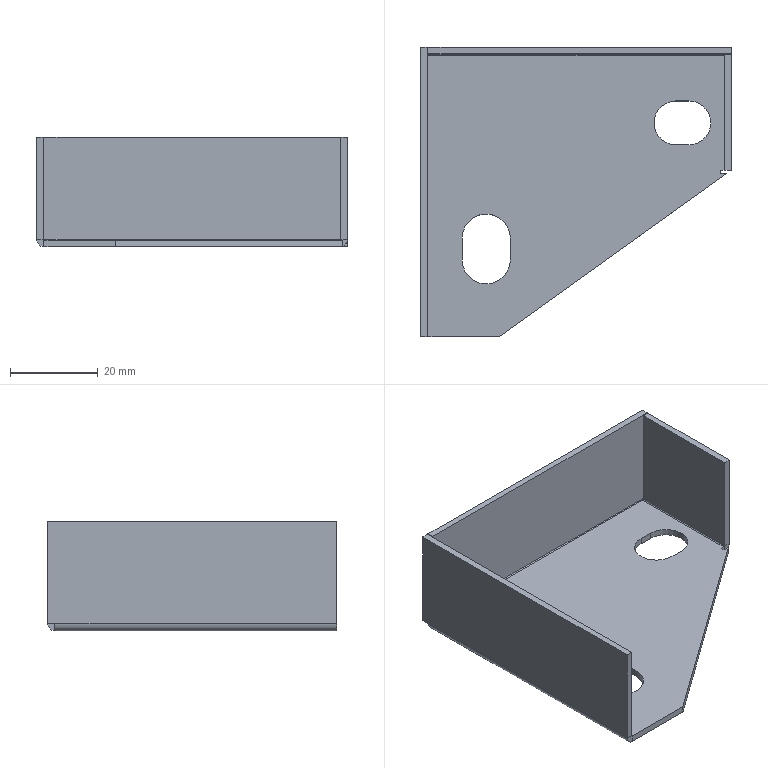Part | 1 solid | 45 faces | box 71 x 66 x 25 mm | volume 10722 mm3 | plane 34 | cylinder 11 | commonest cylinder face diameters 0.4 x3 3.4 x3 10 x3 11 x2
STEP:
#1=CARTESIAN_POINT('',(30.8,15.8,-1.5));
#2=VERTEX_POINT('',#1);
#3=CARTESIAN_POINT('',(25.8,20.8,-1.5));
#4=VERTEX_POINT('',#3);
#5=CARTESIAN_POINT('',(25.8,15.8,-1.5));
#6=DIRECTION('',(0.,0.,1.));
#7=DIRECTION('',(1.,0.,0.));
#8=AXIS2_PLACEMENT_3D('',#5,#6,#7);
#9=CIRCLE('',#8,5.);
#10=EDGE_CURVE('',#2,#4,#9,.T.);
#11=ORIENTED_EDGE('',*,*,#10,.F.);
#12=CARTESIAN_POINT('',(30.8,15.8,0.));
#13=VERTEX_POINT('',#12);
#14=CARTESIAN_POINT('',(30.8,15.8,-10.));
#15=DIRECTION('',(0.,0.,1.));
#16=VECTOR('',#15,1000.);
#17=LINE('',#14,#16);
#18=EDGE_CURVE('',#2,#13,#17,.T.);
#19=ORIENTED_EDGE('',*,*,#18,.T.);
#20=CARTESIAN_POINT('',(25.8,20.8,0.));
#21=VERTEX_POINT('',#20);
#22=CARTESIAN_POINT('',(25.8,15.8,0.));
#23=DIRECTION('',(0.,0.,1.));
#24=DIRECTION('',(1.,0.,0.));
#25=AXIS2_PLACEMENT_3D('',#22,#23,#24);
#26=CIRCLE('',#25,5.);
#27=EDGE_CURVE('',#13,#21,#26,.T.);
#28=ORIENTED_EDGE('',*,*,#27,.T.);
#29=CARTESIAN_POINT('',(25.8,20.8,-10.));
#30=DIRECTION('',(0.,0.,1.));
#31=VECTOR('',#30,1000.);
#32=LINE('',#29,#31);
#33=EDGE_CURVE('',#4,#21,#32,.T.);
#34=ORIENTED_EDGE('',*,*,#33,.F.);
#35=EDGE_LOOP('',(#11,#19,#28,#34));
#36=FACE_OUTER_BOUND('',#35,.T.);
#37=CARTESIAN_POINT('',(25.8,15.8,-10.));
#38=DIRECTION('',(0.,0.,1.));
#39=DIRECTION('',(1.,0.,0.));
#40=AXIS2_PLACEMENT_3D('',#37,#38,#39);
#41=CYLINDRICAL_SURFACE('',#40,5.);
#42=ADVANCED_FACE('',(#36),#41,.F.);
#43=CARTESIAN_POINT('',(35.5,31.3,0.));
#44=VERTEX_POINT('',#43);
#45=CARTESIAN_POINT('',(35.488,31.3,0.));
#46=VERTEX_POINT('',#45);
#47=CARTESIAN_POINT('',(35.5,31.3,0.));
#48=DIRECTION('',(-1.,0.,0.));
#49=VECTOR('',#48,1000.);
#50=LINE('',#47,#49);
#51=EDGE_CURVE('',#44,#46,#50,.T.);
#52=ORIENTED_EDGE('',*,*,#51,.T.);
#53=CARTESIAN_POINT('',(33.8,31.3,-1.5));
#54=VERTEX_POINT('',#53);
#55=CARTESIAN_POINT('',(33.8,31.3,0.2));
#56=DIRECTION('',(0.,1.,0.));
#57=DIRECTION('',(0.,0.,1.));
#58=AXIS2_PLACEMENT_3D('',#55,#56,#57);
#59=CIRCLE('',#58,1.7);
#60=EDGE_CURVE('',#46,#54,#59,.T.);
#61=ORIENTED_EDGE('',*,*,#60,.T.);
#62=CARTESIAN_POINT('',(35.5,31.3,-1.5));
#63=VERTEX_POINT('',#62);
#64=CARTESIAN_POINT('',(-33.8,31.3,-1.5));
#65=DIRECTION('',(-1.,0.,0.));
#66=VECTOR('',#65,1000.);
#67=LINE('',#64,#66);
#68=EDGE_CURVE('',#63,#54,#67,.T.);
#69=ORIENTED_EDGE('',*,*,#68,.F.);
#70=CARTESIAN_POINT('',(35.5,31.3,0.));
#71=DIRECTION('',(0.,0.,-1.));
#72=VECTOR('',#71,1000.);
#73=LINE('',#70,#72);
#74=EDGE_CURVE('',#44,#63,#73,.T.);
#75=ORIENTED_EDGE('',*,*,#74,.F.);
#76=EDGE_LOOP('',(#52,#61,#69,#75));
#77=FACE_OUTER_BOUND('',#76,.T.);
#78=CARTESIAN_POINT('',(35.5,31.3,0.));
#79=DIRECTION('',(0.,-1.,0.));
#80=DIRECTION('',(0.,0.,-1.));
#81=AXIS2_PLACEMENT_3D('',#78,#79,#80);
#82=PLANE('',#81);
#83=ADVANCED_FACE('',(#77),#82,.T.);
#84=CARTESIAN_POINT('',(-15.,-15.5,-1.5));
#85=VERTEX_POINT('',#84);
#86=CARTESIAN_POINT('',(-15.,-10.5,-1.5));
#87=VERTEX_POINT('',#86);
#88=CARTESIAN_POINT('',(-15.,0.,-1.5));
#89=DIRECTION('',(0.,1.,0.));
#90=VECTOR('',#89,1000.);
#91=LINE('',#88,#90);
#92=EDGE_CURVE('',#85,#87,#91,.T.);
#93=ORIENTED_EDGE('',*,*,#92,.T.);
#94=CARTESIAN_POINT('',(-26.,-10.5,-1.5));
#95=VERTEX_POINT('',#94);
#96=CARTESIAN_POINT('',(-20.5,-10.5,-1.5));
#97=DIRECTION('',(0.,0.,1.));
#98=DIRECTION('',(1.,0.,0.));
#99=AXIS2_PLACEMENT_3D('',#96,#97,#98);
#100=CIRCLE('',#99,5.5);
#101=EDGE_CURVE('',#87,#95,#100,.T.);
#102=ORIENTED_EDGE('',*,*,#101,.T.);
#103=CARTESIAN_POINT('',(-26.,-15.5,-1.5));
#104=VERTEX_POINT('',#103);
#105=CARTESIAN_POINT('',(-26.,0.,-1.5));
#106=DIRECTION('',(0.,-1.,0.));
#107=VECTOR('',#106,1000.);
#108=LINE('',#105,#107);
#109=EDGE_CURVE('',#95,#104,#108,.T.);
#110=ORIENTED_EDGE('',*,*,#109,.T.);
#111=CARTESIAN_POINT('',(-20.5,-15.5,-1.5));
#112=DIRECTION('',(0.,0.,1.));
#113=DIRECTION('',(1.,0.,0.));
#114=AXIS2_PLACEMENT_3D('',#111,#112,#113);
#115=CIRCLE('',#114,5.5);
#116=EDGE_CURVE('',#104,#85,#115,.T.);
#117=ORIENTED_EDGE('',*,*,#116,.T.);
#118=EDGE_LOOP('',(#93,#102,#110,#117));
#119=FACE_BOUND('',#118,.T.);
#120=CARTESIAN_POINT('',(22.8,20.8,-1.5));
#121=VERTEX_POINT('',#120);
#122=CARTESIAN_POINT('',(0.,20.8,-1.5));
#123=DIRECTION('',(-1.,0.,0.));
#124=VECTOR('',#123,1000.);
#125=LINE('',#122,#124);
#126=EDGE_CURVE('',#4,#121,#125,.T.);
#127=ORIENTED_EDGE('',*,*,#126,.T.);
#128=CARTESIAN_POINT('',(22.8,10.8,-1.5));
#129=VERTEX_POINT('',#128);
#130=CARTESIAN_POINT('',(22.8,15.8,-1.5));
#131=DIRECTION('',(0.,0.,1.));
#132=DIRECTION('',(1.,0.,0.));
#133=AXIS2_PLACEMENT_3D('',#130,#131,#132);
#134=CIRCLE('',#133,5.);
#135=EDGE_CURVE('',#121,#129,#134,.T.);
#136=ORIENTED_EDGE('',*,*,#135,.T.);
#137=CARTESIAN_POINT('',(25.8,10.8,-1.5));
#138=VERTEX_POINT('',#137);
#139=CARTESIAN_POINT('',(0.,10.8,-1.5));
#140=DIRECTION('',(1.,0.,0.));
#141=VECTOR('',#140,1000.);
#142=LINE('',#139,#141);
#143=EDGE_CURVE('',#129,#138,#142,.T.);
#144=ORIENTED_EDGE('',*,*,#143,.T.);
#145=CARTESIAN_POINT('',(25.8,15.8,-1.5));
#146=DIRECTION('',(0.,0.,1.));
#147=DIRECTION('',(1.,0.,0.));
#148=AXIS2_PLACEMENT_3D('',#145,#146,#147);
#149=CIRCLE('',#148,5.);
#150=EDGE_CURVE('',#138,#2,#149,.T.);
#151=ORIENTED_EDGE('',*,*,#150,.T.);
#152=ORIENTED_EDGE('',*,*,#10,.T.);
#153=EDGE_LOOP('',(#127,#136,#144,#151,#152));
#154=FACE_BOUND('',#153,.T.);
#155=CARTESIAN_POINT('',(33.8,5.,-1.5));
#156=VERTEX_POINT('',#155);
#157=CARTESIAN_POINT('',(33.8,31.3,-1.5));
#158=DIRECTION('',(0.,-1.,0.));
#159=VECTOR('',#158,1000.);
#160=LINE('',#157,#159);
#161=EDGE_CURVE('',#54,#156,#160,.T.);
#162=ORIENTED_EDGE('',*,*,#161,.T.);
#163=CARTESIAN_POINT('',(33.05,5.,-1.5));
#164=VERTEX_POINT('',#163);
#165=CARTESIAN_POINT('',(0.,5.,-1.5));
#166=DIRECTION('',(1.,0.,0.));
#167=VECTOR('',#166,1000.);
#168=LINE('',#165,#167);
#169=EDGE_CURVE('',#164,#156,#168,.T.);
#170=ORIENTED_EDGE('',*,*,#169,.F.);
#171=CARTESIAN_POINT('',(33.05,4.25,-1.5));
#172=VERTEX_POINT('',#171);
#173=CARTESIAN_POINT('',(33.05,0.,-1.5));
#174=DIRECTION('',(0.,1.,0.));
#175=VECTOR('',#174,1000.);
#176=LINE('',#173,#175);
#177=EDGE_CURVE('',#172,#164,#176,.T.);
#178=ORIENTED_EDGE('',*,*,#177,.F.);
#179=CARTESIAN_POINT('',(34.454,4.25,-1.5));
#180=VERTEX_POINT('',#179);
#181=CARTESIAN_POINT('',(0.,4.25,-1.5));
#182=DIRECTION('',(-1.,0.,0.));
#183=VECTOR('',#182,1000.);
#184=LINE('',#181,#183);
#185=EDGE_CURVE('',#180,#172,#184,.T.);
#186=ORIENTED_EDGE('',*,*,#185,.F.);
#187=CARTESIAN_POINT('',(-17.5,-33.,-1.5));
#188=VERTEX_POINT('',#187);
#189=CARTESIAN_POINT('',(9.685,-13.509,-1.5));
#190=DIRECTION('',(-0.8127,-0.5827,0.));
#191=VECTOR('',#190,1000.);
#192=LINE('',#189,#191);
#193=EDGE_CURVE('',#180,#188,#192,.T.);
#194=ORIENTED_EDGE('',*,*,#193,.T.);
#195=CARTESIAN_POINT('',(-33.8,-33.,-1.5));
#196=VERTEX_POINT('',#195);
#197=CARTESIAN_POINT('',(-35.5,-33.,-1.5));
#198=DIRECTION('',(1.,0.,0.));
#199=VECTOR('',#198,1000.);
#200=LINE('',#197,#199);
#201=EDGE_CURVE('',#196,#188,#200,.T.);
#202=ORIENTED_EDGE('',*,*,#201,.F.);
#203=CARTESIAN_POINT('',(-33.8,31.3,-1.5));
#204=VERTEX_POINT('',#203);
#205=CARTESIAN_POINT('',(-33.8,-33.,-1.5));
#206=DIRECTION('',(0.,1.,0.));
#207=VECTOR('',#206,1000.);
#208=LINE('',#205,#207);
#209=EDGE_CURVE('',#196,#204,#208,.T.);
#210=ORIENTED_EDGE('',*,*,#209,.T.);
#211=CARTESIAN_POINT('',(-33.8,31.3,-1.5));
#212=DIRECTION('',(1.,0.,0.));
#213=VECTOR('',#212,1000.);
#214=LINE('',#211,#213);
#215=EDGE_CURVE('',#204,#54,#214,.T.);
#216=ORIENTED_EDGE('',*,*,#215,.T.);
#217=EDGE_LOOP('',(#162,#170,#178,#186,#194,#202,#210,#216));
#218=FACE_OUTER_BOUND('',#217,.T.);
#219=CARTESIAN_POINT('',(0.,0.,-1.5));
#220=DIRECTION('',(0.,0.,1.));
#221=DIRECTION('',(1.,0.,0.));
#222=AXIS2_PLACEMENT_3D('',#219,#220,#221);
#223=PLANE('',#222);
#224=ADVANCED_FACE('',(#119,#154,#218),#223,.F.);
#225=CARTESIAN_POINT('',(22.8,20.8,0.));
#226=VERTEX_POINT('',#225);
#227=CARTESIAN_POINT('',(22.8,10.8,0.));
#228=VERTEX_POINT('',#227);
#229=CARTESIAN_POINT('',(22.8,15.8,0.));
#230=DIRECTION('',(0.,0.,1.));
#231=DIRECTION('',(1.,0.,0.));
#232=AXIS2_PLACEMENT_3D('',#229,#230,#231);
#233=CIRCLE('',#232,5.);
#234=EDGE_CURVE('',#226,#228,#233,.T.);
#235=ORIENTED_EDGE('',*,*,#234,.F.);
#236=CARTESIAN_POINT('',(22.8,20.8,0.));
#237=DIRECTION('',(-1.,0.,0.));
#238=VECTOR('',#237,1000.);
#239=LINE('',#236,#238);
#240=EDGE_CURVE('',#21,#226,#239,.T.);
#241=ORIENTED_EDGE('',*,*,#240,.F.);
#242=ORIENTED_EDGE('',*,*,#27,.F.);
#243=CARTESIAN_POINT('',(25.8,10.8,0.));
#244=VERTEX_POINT('',#243);
#245=CARTESIAN_POINT('',(25.8,15.8,0.));
#246=DIRECTION('',(0.,0.,1.));
#247=DIRECTION('',(1.,0.,0.));
#248=AXIS2_PLACEMENT_3D('',#245,#246,#247);
#249=CIRCLE('',#248,5.);
#250=EDGE_CURVE('',#244,#13,#249,.T.);
#251=ORIENTED_EDGE('',*,*,#250,.F.);
#252=CARTESIAN_POINT('',(22.8,10.8,0.));
#253=DIRECTION('',(1.,0.,0.));
#254=VECTOR('',#253,1000.);
#255=LINE('',#252,#254);
#256=EDGE_CURVE('',#228,#244,#255,.T.);
#257=ORIENTED_EDGE('',*,*,#256,.F.);
#258=EDGE_LOOP('',(#235,#241,#242,#251,#257));
#259=FACE_BOUND('',#258,.T.);
#260=CARTESIAN_POINT('',(-15.,-10.5,0.));
#261=VERTEX_POINT('',#260);
#262=CARTESIAN_POINT('',(-26.,-10.5,0.));
#263=VERTEX_POINT('',#262);
#264=CARTESIAN_POINT('',(-20.5,-10.5,0.));
#265=DIRECTION('',(0.,0.,1.));
#266=DIRECTION('',(1.,0.,0.));
#267=AXIS2_PLACEMENT_3D('',#264,#265,#266);
#268=CIRCLE('',#267,5.5);
#269=EDGE_CURVE('',#261,#263,#268,.T.);
#270=ORIENTED_EDGE('',*,*,#269,.F.);
#271=CARTESIAN_POINT('',(-15.,-15.5,0.));
#272=VERTEX_POINT('',#271);
#273=CARTESIAN_POINT('',(-15.,-10.5,0.));
#274=DIRECTION('',(0.,1.,0.));
#275=VECTOR('',#274,1000.);
#276=LINE('',#273,#275);
#277=EDGE_CURVE('',#272,#261,#276,.T.);
#278=ORIENTED_EDGE('',*,*,#277,.F.);
#279=CARTESIAN_POINT('',(-26.,-15.5,0.));
#280=VERTEX_POINT('',#279);
#281=CARTESIAN_POINT('',(-20.5,-15.5,0.));
#282=DIRECTION('',(0.,0.,1.));
#283=DIRECTION('',(1.,0.,0.));
#284=AXIS2_PLACEMENT_3D('',#281,#282,#283);
#285=CIRCLE('',#284,5.5);
#286=EDGE_CURVE('',#280,#272,#285,.T.);
#287=ORIENTED_EDGE('',*,*,#286,.F.);
#288=CARTESIAN_POINT('',(-26.,-10.5,0.));
#289=DIRECTION('',(0.,-1.,0.));
#290=VECTOR('',#289,1000.);
#291=LINE('',#288,#290);
#292=EDGE_CURVE('',#263,#280,#291,.T.);
#293=ORIENTED_EDGE('',*,*,#292,.F.);
#294=EDGE_LOOP('',(#270,#278,#287,#293));
#295=FACE_BOUND('',#294,.T.);
#296=CARTESIAN_POINT('',(33.8,5.,0.));
#297=VERTEX_POINT('',#296);
#298=CARTESIAN_POINT('',(33.05,5.,0.));
#299=VERTEX_POINT('',#298);
#300=CARTESIAN_POINT('',(33.8,5.,0.));
#301=DIRECTION('',(-1.,0.,0.));
#302=VECTOR('',#301,1000.);
#303=LINE('',#300,#302);
#304=EDGE_CURVE('',#297,#299,#303,.T.);
#305=ORIENTED_EDGE('',*,*,#304,.F.);
#306=CARTESIAN_POINT('',(33.8,31.3,0.));
#307=VERTEX_POINT('',#306);
#308=CARTESIAN_POINT('',(33.8,31.3,0.));
#309=DIRECTION('',(0.,-1.,0.));
#310=VECTOR('',#309,1000.);
#311=LINE('',#308,#310);
#312=EDGE_CURVE('',#307,#297,#311,.T.);
#313=ORIENTED_EDGE('',*,*,#312,.F.);
#314=CARTESIAN_POINT('',(-33.8,31.3,0.));
#315=VERTEX_POINT('',#314);
#316=CARTESIAN_POINT('',(-33.8,31.3,0.));
#317=DIRECTION('',(1.,0.,0.));
#318=VECTOR('',#317,1000.);
#319=LINE('',#316,#318);
#320=EDGE_CURVE('',#315,#307,#319,.T.);
#321=ORIENTED_EDGE('',*,*,#320,.F.);
#322=CARTESIAN_POINT('',(-33.8,-33.,0.));
#323=VERTEX_POINT('',#322);
#324=CARTESIAN_POINT('',(-33.8,-33.,0.));
#325=DIRECTION('',(0.,1.,0.));
#326=VECTOR('',#325,1000.);
#327=LINE('',#324,#326);
#328=EDGE_CURVE('',#323,#315,#327,.T.);
#329=ORIENTED_EDGE('',*,*,#328,.F.);
#330=CARTESIAN_POINT('',(-17.5,-33.,0.));
#331=VERTEX_POINT('',#330);
#332=CARTESIAN_POINT('',(-35.5,-33.,0.));
#333=DIRECTION('',(1.,0.,0.));
#334=VECTOR('',#333,1000.);
#335=LINE('',#332,#334);
#336=EDGE_CURVE('',#323,#331,#335,.T.);
#337=ORIENTED_EDGE('',*,*,#336,.T.);
#338=CARTESIAN_POINT('',(34.454,4.25,0.));
#339=VERTEX_POINT('',#338);
#340=CARTESIAN_POINT('',(9.685,-13.509,0.));
#341=DIRECTION('',(-0.8127,-0.5827,0.));
#342=VECTOR('',#341,1000.);
#343=LINE('',#340,#342);
#344=EDGE_CURVE('',#339,#331,#343,.T.);
#345=ORIENTED_EDGE('',*,*,#344,.F.);
#346=CARTESIAN_POINT('',(33.05,4.25,0.));
#347=VERTEX_POINT('',#346);
#348=CARTESIAN_POINT('',(33.05,4.25,0.));
#349=DIRECTION('',(1.,0.,0.));
#350=VECTOR('',#349,1000.);
#351=LINE('',#348,#350);
#352=EDGE_CURVE('',#347,#339,#351,.T.);
#353=ORIENTED_EDGE('',*,*,#352,.F.);
#354=CARTESIAN_POINT('',(33.05,5.,0.));
#355=DIRECTION('',(0.,-1.,0.));
#356=VECTOR('',#355,1000.);
#357=LINE('',#354,#356);
#358=EDGE_CURVE('',#299,#347,#357,.T.);
#359=ORIENTED_EDGE('',*,*,#358,.F.);
#360=EDGE_LOOP('',(#305,#313,#321,#329,#337,#345,#353,#359));
#361=FACE_OUTER_BOUND('',#360,.T.);
#362=CARTESIAN_POINT('',(0.,0.,0.));
#363=DIRECTION('',(0.,0.,1.));
#364=DIRECTION('',(1.,0.,0.));
#365=AXIS2_PLACEMENT_3D('',#362,#363,#364);
#366=PLANE('',#365);
#367=ADVANCED_FACE('',(#259,#295,#361),#366,.T.);
#368=CARTESIAN_POINT('',(34.454,4.25,0.));
#369=DIRECTION('',(0.,0.,-1.));
#370=VECTOR('',#369,1000.);
#371=LINE('',#368,#370);
#372=EDGE_CURVE('',#339,#180,#371,.T.);
#373=ORIENTED_EDGE('',*,*,#372,.F.);
#374=ORIENTED_EDGE('',*,*,#344,.T.);
#375=CARTESIAN_POINT('',(-17.5,-33.,23.5));
#376=DIRECTION('',(0.,0.,-1.));
#377=VECTOR('',#376,1000.);
#378=LINE('',#375,#377);
#379=EDGE_CURVE('',#331,#188,#378,.T.);
#380=ORIENTED_EDGE('',*,*,#379,.T.);
#381=ORIENTED_EDGE('',*,*,#193,.F.);
#382=EDGE_LOOP('',(#373,#374,#380,#381));
#383=FACE_OUTER_BOUND('',#382,.T.);
#384=CARTESIAN_POINT('',(35.5,5.,23.5));
#385=DIRECTION('',(-0.5827,0.8127,0.));
#386=DIRECTION('',(-0.8127,-0.5827,0.));
#387=AXIS2_PLACEMENT_3D('',#384,#385,#386);
#388=PLANE('',#387);
#389=ADVANCED_FACE('',(#383),#388,.F.);
#390=CARTESIAN_POINT('',(-35.5,31.3,0.2));
#391=VERTEX_POINT('',#390);
#392=CARTESIAN_POINT('',(-34.,31.3,0.2));
#393=VERTEX_POINT('',#392);
#394=CARTESIAN_POINT('',(-35.5,31.3,0.2));
#395=DIRECTION('',(1.,0.,0.));
#396=VECTOR('',#395,1000.);
#397=LINE('',#394,#396);
#398=EDGE_CURVE('',#391,#393,#397,.T.);
#399=ORIENTED_EDGE('',*,*,#398,.F.);
#400=CARTESIAN_POINT('',(-35.5,33.,0.2));
#401=VERTEX_POINT('',#400);
#402=CARTESIAN_POINT('',(-35.5,33.,0.2));
#403=DIRECTION('',(0.,1.,0.));
#404=VECTOR('',#403,1000.);
#405=LINE('',#402,#404);
#406=EDGE_CURVE('',#391,#401,#405,.T.);
#407=ORIENTED_EDGE('',*,*,#406,.T.);
#408=CARTESIAN_POINT('',(-34.,33.,0.2));
#409=VERTEX_POINT('',#408);
#410=CARTESIAN_POINT('',(-35.5,33.,0.2));
#411=DIRECTION('',(-1.,0.,0.));
#412=VECTOR('',#411,1000.);
#413=LINE('',#410,#412);
#414=EDGE_CURVE('',#409,#401,#413,.T.);
#415=ORIENTED_EDGE('',*,*,#414,.F.);
#416=CARTESIAN_POINT('',(-34.,33.,0.2));
#417=DIRECTION('',(0.,-1.,0.));
#418=VECTOR('',#417,1000.);
#419=LINE('',#416,#418);
#420=EDGE_CURVE('',#409,#393,#419,.T.);
#421=ORIENTED_EDGE('',*,*,#420,.T.);
#422=EDGE_LOOP('',(#399,#407,#415,#421));
#423=FACE_OUTER_BOUND('',#422,.T.);
#424=CARTESIAN_POINT('',(0.,0.,0.2));
#425=DIRECTION('',(0.,0.,-1.));
#426=DIRECTION('',(-1.,0.,0.));
#427=AXIS2_PLACEMENT_3D('',#424,#425,#426);
#428=PLANE('',#427);
#429=ADVANCED_FACE('',(#423),#428,.T.);
#430=CARTESIAN_POINT('',(-35.5,-33.,0.2));
#431=VERTEX_POINT('',#430);
#432=CARTESIAN_POINT('',(-35.5,33.,0.2));
#433=DIRECTION('',(0.,1.,0.));
#434=VECTOR('',#433,1000.);
#435=LINE('',#432,#434);
#436=EDGE_CURVE('',#431,#391,#435,.T.);
#437=ORIENTED_EDGE('',*,*,#436,.T.);
#438=CARTESIAN_POINT('',(-33.8,31.3,0.2));
#439=DIRECTION('',(0.,-1.,0.));
#440=DIRECTION('',(0.,0.,1.));
#441=AXIS2_PLACEMENT_3D('',#438,#439,#440);
#442=CIRCLE('',#441,1.7);
#443=EDGE_CURVE('',#391,#204,#442,.T.);
#444=ORIENTED_EDGE('',*,*,#443,.T.);
#445=ORIENTED_EDGE('',*,*,#209,.F.);
#446=CARTESIAN_POINT('',(-33.8,-33.,0.2));
#447=DIRECTION('',(0.,-1.,0.));
#448=DIRECTION('',(0.,0.,-1.));
#449=AXIS2_PLACEMENT_3D('',#446,#447,#448);
#450=CIRCLE('',#449,1.7);
#451=EDGE_CURVE('',#431,#196,#450,.T.);
#452=ORIENTED_EDGE('',*,*,#451,.F.);
#453=EDGE_LOOP('',(#437,#444,#445,#452));
#454=FACE_OUTER_BOUND('',#453,.T.);
#455=CARTESIAN_POINT('',(-33.8,-33.,0.2));
#456=DIRECTION('',(0.,-1.,0.));
#457=DIRECTION('',(-1.,0.,0.));
#458=AXIS2_PLACEMENT_3D('',#455,#456,#457);
#459=CYLINDRICAL_SURFACE('',#458,1.7);
#460=ADVANCED_FACE('',(#454),#459,.T.);
#461=ORIENTED_EDGE('',*,*,#379,.F.);
#462=ORIENTED_EDGE('',*,*,#336,.F.);
#463=CARTESIAN_POINT('',(-33.8,-33.,0.));
#464=DIRECTION('',(0.,0.,-1.));
#465=VECTOR('',#464,1000.);
#466=LINE('',#463,#465);
#467=EDGE_CURVE('',#323,#196,#466,.T.);
#468=ORIENTED_EDGE('',*,*,#467,.T.);
#469=ORIENTED_EDGE('',*,*,#201,.T.);
#470=EDGE_LOOP('',(#461,#462,#468,#469));
#471=FACE_OUTER_BOUND('',#470,.T.);
#472=CARTESIAN_POINT('',(-35.5,-33.,-1.5));
#473=DIRECTION('',(0.,-1.,0.));
#474=DIRECTION('',(0.,0.,-1.));
#475=AXIS2_PLACEMENT_3D('',#472,#473,#474);
#476=PLANE('',#475);
#477=ADVANCED_FACE('',(#471),#476,.T.);
#478=CARTESIAN_POINT('',(-15.,-10.5,-10.));
#479=DIRECTION('',(0.,0.,1.));
#480=VECTOR('',#479,1000.);
#481=LINE('',#478,#480);
#482=EDGE_CURVE('',#87,#261,#481,.T.);
#483=ORIENTED_EDGE('',*,*,#482,.T.);
#484=ORIENTED_EDGE('',*,*,#269,.T.);
#485=CARTESIAN_POINT('',(-26.,-10.5,-10.));
#486=DIRECTION('',(0.,0.,1.));
#487=VECTOR('',#486,1000.);
#488=LINE('',#485,#487);
#489=EDGE_CURVE('',#95,#263,#488,.T.);
#490=ORIENTED_EDGE('',*,*,#489,.F.);
#491=ORIENTED_EDGE('',*,*,#101,.F.);
#492=EDGE_LOOP('',(#483,#484,#490,#491));
#493=FACE_OUTER_BOUND('',#492,.T.);
#494=CARTESIAN_POINT('',(-20.5,-10.5,-10.));
#495=DIRECTION('',(0.,0.,1.));
#496=DIRECTION('',(1.,0.,0.));
#497=AXIS2_PLACEMENT_3D('',#494,#495,#496);
#498=CYLINDRICAL_SURFACE('',#497,5.5);
#499=ADVANCED_FACE('',(#493),#498,.F.);
#500=CARTESIAN_POINT('',(-15.,-15.5,-10.));
#501=DIRECTION('',(0.,0.,1.));
#502=VECTOR('',#501,1000.);
#503=LINE('',#500,#502);
#504=EDGE_CURVE('',#85,#272,#503,.T.);
#505=ORIENTED_EDGE('',*,*,#504,.T.);
#506=ORIENTED_EDGE('',*,*,#277,.T.);
#507=ORIENTED_EDGE('',*,*,#482,.F.);
#508=ORIENTED_EDGE('',*,*,#92,.F.);
#509=EDGE_LOOP('',(#505,#506,#507,#508));
#510=FACE_OUTER_BOUND('',#509,.T.);
#511=CARTESIAN_POINT('',(-15.,-10.5,-10.));
#512=DIRECTION('',(1.,0.,0.));
#513=DIRECTION('',(0.,0.,-1.));
#514=AXIS2_PLACEMENT_3D('',#511,#512,#513);
#515=PLANE('',#514);
#516=ADVANCED_FACE('',(#510),#515,.F.);
#517=CARTESIAN_POINT('',(-26.,-15.5,-10.));
#518=DIRECTION('',(0.,0.,1.));
#519=VECTOR('',#518,1000.);
#520=LINE('',#517,#519);
#521=EDGE_CURVE('',#104,#280,#520,.T.);
#522=ORIENTED_EDGE('',*,*,#521,.T.);
#523=ORIENTED_EDGE('',*,*,#286,.T.);
#524=ORIENTED_EDGE('',*,*,#504,.F.);
#525=ORIENTED_EDGE('',*,*,#116,.F.);
#526=EDGE_LOOP('',(#522,#523,#524,#525));
#527=FACE_OUTER_BOUND('',#526,.T.);
#528=CARTESIAN_POINT('',(-20.5,-15.5,-10.));
#529=DIRECTION('',(0.,0.,1.));
#530=DIRECTION('',(1.,0.,0.));
#531=AXIS2_PLACEMENT_3D('',#528,#529,#530);
#532=CYLINDRICAL_SURFACE('',#531,5.5);
#533=ADVANCED_FACE('',(#527),#532,.F.);
#534=ORIENTED_EDGE('',*,*,#489,.T.);
#535=ORIENTED_EDGE('',*,*,#292,.T.);
#536=ORIENTED_EDGE('',*,*,#521,.F.);
#537=ORIENTED_EDGE('',*,*,#109,.F.);
#538=EDGE_LOOP('',(#534,#535,#536,#537));
#539=FACE_OUTER_BOUND('',#538,.T.);
#540=CARTESIAN_POINT('',(-26.,-10.5,-10.));
#541=DIRECTION('',(-1.,0.,0.));
#542=DIRECTION('',(0.,0.,1.));
#543=AXIS2_PLACEMENT_3D('',#540,#541,#542);
#544=PLANE('',#543);
#545=ADVANCED_FACE('',(#539),#544,.F.);
#546=CARTESIAN_POINT('',(22.8,20.8,-10.));
#547=DIRECTION('',(0.,0.,1.));
#548=VECTOR('',#547,1000.);
#549=LINE('',#546,#548);
#550=EDGE_CURVE('',#121,#226,#549,.T.);
#551=ORIENTED_EDGE('',*,*,#550,.T.);
#552=ORIENTED_EDGE('',*,*,#234,.T.);
#553=CARTESIAN_POINT('',(22.8,10.8,-10.));
#554=DIRECTION('',(0.,0.,1.));
#555=VECTOR('',#554,1000.);
#556=LINE('',#553,#555);
#557=EDGE_CURVE('',#129,#228,#556,.T.);
#558=ORIENTED_EDGE('',*,*,#557,.F.);
#559=ORIENTED_EDGE('',*,*,#135,.F.);
#560=EDGE_LOOP('',(#551,#552,#558,#559));
#561=FACE_OUTER_BOUND('',#560,.T.);
#562=CARTESIAN_POINT('',(22.8,15.8,-10.));
#563=DIRECTION('',(0.,0.,1.));
#564=DIRECTION('',(1.,0.,0.));
#565=AXIS2_PLACEMENT_3D('',#562,#563,#564);
#566=CYLINDRICAL_SURFACE('',#565,5.);
#567=ADVANCED_FACE('',(#561),#566,.F.);
#568=ORIENTED_EDGE('',*,*,#33,.T.);
#569=ORIENTED_EDGE('',*,*,#240,.T.);
#570=ORIENTED_EDGE('',*,*,#550,.F.);
#571=ORIENTED_EDGE('',*,*,#126,.F.);
#572=EDGE_LOOP('',(#568,#569,#570,#571));
#573=FACE_OUTER_BOUND('',#572,.T.);
#574=CARTESIAN_POINT('',(22.8,20.8,-10.));
#575=DIRECTION('',(0.,1.,0.));
#576=DIRECTION('',(0.,0.,1.));
#577=AXIS2_PLACEMENT_3D('',#574,#575,#576);
#578=PLANE('',#577);
#579=ADVANCED_FACE('',(#573),#578,.F.);
#580=ORIENTED_EDGE('',*,*,#18,.F.);
#581=ORIENTED_EDGE('',*,*,#150,.F.);
#582=CARTESIAN_POINT('',(25.8,10.8,-10.));
#583=DIRECTION('',(0.,0.,1.));
#584=VECTOR('',#583,1000.);
#585=LINE('',#582,#584);
#586=EDGE_CURVE('',#138,#244,#585,.T.);
#587=ORIENTED_EDGE('',*,*,#586,.T.);
#588=ORIENTED_EDGE('',*,*,#250,.T.);
#589=EDGE_LOOP('',(#580,#581,#587,#588));
#590=FACE_OUTER_BOUND('',#589,.T.);
#591=CARTESIAN_POINT('',(25.8,15.8,-10.));
#592=DIRECTION('',(0.,0.,1.));
#593=DIRECTION('',(1.,0.,0.));
#594=AXIS2_PLACEMENT_3D('',#591,#592,#593);
#595=CYLINDRICAL_SURFACE('',#594,5.);
#596=ADVANCED_FACE('',(#590),#595,.F.);
#597=ORIENTED_EDGE('',*,*,#557,.T.);
#598=ORIENTED_EDGE('',*,*,#256,.T.);
#599=ORIENTED_EDGE('',*,*,#586,.F.);
#600=ORIENTED_EDGE('',*,*,#143,.F.);
#601=EDGE_LOOP('',(#597,#598,#599,#600));
#602=FACE_OUTER_BOUND('',#601,.T.);
#603=CARTESIAN_POINT('',(22.8,10.8,-10.));
#604=DIRECTION('',(0.,-1.,0.));
#605=DIRECTION('',(0.,0.,-1.));
#606=AXIS2_PLACEMENT_3D('',#603,#604,#605);
#607=PLANE('',#606);
#608=ADVANCED_FACE('',(#602),#607,.F.);
#609=CARTESIAN_POINT('',(-34.,-33.,0.2));
#610=VERTEX_POINT('',#609);
#611=CARTESIAN_POINT('',(-33.8,-33.,0.2));
#612=DIRECTION('',(0.,-1.,0.));
#613=DIRECTION('',(0.,0.,-1.));
#614=AXIS2_PLACEMENT_3D('',#611,#612,#613);
#615=CIRCLE('',#614,0.2);
#616=EDGE_CURVE('',#610,#323,#615,.T.);
#617=ORIENTED_EDGE('',*,*,#616,.F.);
#618=CARTESIAN_POINT('',(-34.,-33.,0.2));
#619=DIRECTION('',(-1.,0.,0.));
#620=VECTOR('',#619,1000.);
#621=LINE('',#618,#620);
#622=EDGE_CURVE('',#610,#431,#621,.T.);
#623=ORIENTED_EDGE('',*,*,#622,.T.);
#624=ORIENTED_EDGE('',*,*,#451,.T.);
#625=ORIENTED_EDGE('',*,*,#467,.F.);
#626=EDGE_LOOP('',(#617,#623,#624,#625));
#627=FACE_OUTER_BOUND('',#626,.T.);
#628=CARTESIAN_POINT('',(-33.8,-33.,0.2));
#629=DIRECTION('',(0.,1.,0.));
#630=DIRECTION('',(0.,0.,1.));
#631=AXIS2_PLACEMENT_3D('',#628,#629,#630);
#632=PLANE('',#631);
#633=ADVANCED_FACE('',(#627),#632,.F.);
#634=ORIENTED_EDGE('',*,*,#443,.F.);
#635=ORIENTED_EDGE('',*,*,#398,.T.);
#636=CARTESIAN_POINT('',(-33.8,31.3,0.2));
#637=DIRECTION('',(0.,-1.,0.));
#638=DIRECTION('',(0.,0.,1.));
#639=AXIS2_PLACEMENT_3D('',#636,#637,#638);
#640=CIRCLE('',#639,0.2);
#641=EDGE_CURVE('',#393,#315,#640,.T.);
#642=ORIENTED_EDGE('',*,*,#641,.T.);
#643=CARTESIAN_POINT('',(-33.8,31.3,0.));
#644=DIRECTION('',(0.,0.,-1.));
#645=VECTOR('',#644,1000.);
#646=LINE('',#643,#645);
#647=EDGE_CURVE('',#315,#204,#646,.T.);
#648=ORIENTED_EDGE('',*,*,#647,.T.);
#649=EDGE_LOOP('',(#634,#635,#642,#648));
#650=FACE_OUTER_BOUND('',#649,.T.);
#651=CARTESIAN_POINT('',(-33.8,31.3,0.2));
#652=DIRECTION('',(0.,1.,0.));
#653=DIRECTION('',(0.,0.,1.));
#654=AXIS2_PLACEMENT_3D('',#651,#652,#653);
#655=PLANE('',#654);
#656=ADVANCED_FACE('',(#650),#655,.T.);
#657=ORIENTED_EDGE('',*,*,#641,.F.);
#658=CARTESIAN_POINT('',(-34.,33.,0.2));
#659=DIRECTION('',(0.,-1.,0.));
#660=VECTOR('',#659,1000.);
#661=LINE('',#658,#660);
#662=EDGE_CURVE('',#393,#610,#661,.T.);
#663=ORIENTED_EDGE('',*,*,#662,.T.);
#664=ORIENTED_EDGE('',*,*,#616,.T.);
#665=ORIENTED_EDGE('',*,*,#328,.T.);
#666=EDGE_LOOP('',(#657,#663,#664,#665));
#667=FACE_OUTER_BOUND('',#666,.T.);
#668=CARTESIAN_POINT('',(-33.8,-33.,0.2));
#669=DIRECTION('',(0.,-1.,0.));
#670=DIRECTION('',(-1.,0.,0.));
#671=AXIS2_PLACEMENT_3D('',#668,#669,#670);
#672=CYLINDRICAL_SURFACE('',#671,0.2);
#673=ADVANCED_FACE('',(#667),#672,.F.);
#674=ORIENTED_EDGE('',*,*,#414,.T.);
#675=CARTESIAN_POINT('',(-35.5,33.,23.5));
#676=VERTEX_POINT('',#675);
#677=CARTESIAN_POINT('',(-35.5,33.,0.));
#678=DIRECTION('',(0.,0.,-1.));
#679=VECTOR('',#678,1000.);
#680=LINE('',#677,#679);
#681=EDGE_CURVE('',#676,#401,#680,.T.);
#682=ORIENTED_EDGE('',*,*,#681,.F.);
#683=CARTESIAN_POINT('',(-34.,33.,23.5));
#684=VERTEX_POINT('',#683);
#685=CARTESIAN_POINT('',(-35.5,33.,23.5));
#686=DIRECTION('',(1.,0.,0.));
#687=VECTOR('',#686,1000.);
#688=LINE('',#685,#687);
#689=EDGE_CURVE('',#676,#684,#688,.T.);
#690=ORIENTED_EDGE('',*,*,#689,.T.);
#691=CARTESIAN_POINT('',(-34.,33.,0.));
#692=DIRECTION('',(0.,0.,-1.));
#693=VECTOR('',#692,1000.);
#694=LINE('',#691,#693);
#695=EDGE_CURVE('',#684,#409,#694,.T.);
#696=ORIENTED_EDGE('',*,*,#695,.T.);
#697=EDGE_LOOP('',(#674,#682,#690,#696));
#698=FACE_OUTER_BOUND('',#697,.T.);
#699=CARTESIAN_POINT('',(-35.5,33.,0.));
#700=DIRECTION('',(0.,-1.,0.));
#701=DIRECTION('',(1.,0.,0.));
#702=AXIS2_PLACEMENT_3D('',#699,#700,#701);
#703=PLANE('',#702);
#704=ADVANCED_FACE('',(#698),#703,.F.);
#705=ORIENTED_EDGE('',*,*,#622,.F.);
#706=CARTESIAN_POINT('',(-34.,-33.,23.5));
#707=VERTEX_POINT('',#706);
#708=CARTESIAN_POINT('',(-34.,-33.,23.5));
#709=DIRECTION('',(0.,0.,1.));
#710=VECTOR('',#709,1000.);
#711=LINE('',#708,#710);
#712=EDGE_CURVE('',#610,#707,#711,.T.);
#713=ORIENTED_EDGE('',*,*,#712,.T.);
#714=CARTESIAN_POINT('',(-35.5,-33.,23.5));
#715=VERTEX_POINT('',#714);
#716=CARTESIAN_POINT('',(-35.5,-33.,23.5));
#717=DIRECTION('',(1.,0.,0.));
#718=VECTOR('',#717,1000.);
#719=LINE('',#716,#718);
#720=EDGE_CURVE('',#715,#707,#719,.T.);
#721=ORIENTED_EDGE('',*,*,#720,.F.);
#722=CARTESIAN_POINT('',(-35.5,-33.,0.));
#723=DIRECTION('',(0.,0.,1.));
#724=VECTOR('',#723,1000.);
#725=LINE('',#722,#724);
#726=EDGE_CURVE('',#431,#715,#725,.T.);
#727=ORIENTED_EDGE('',*,*,#726,.F.);
#728=EDGE_LOOP('',(#705,#713,#721,#727));
#729=FACE_OUTER_BOUND('',#728,.T.);
#730=CARTESIAN_POINT('',(-35.5,-33.,23.5));
#731=DIRECTION('',(0.,1.,0.));
#732=DIRECTION('',(-1.,0.,0.));
#733=AXIS2_PLACEMENT_3D('',#730,#731,#732);
#734=PLANE('',#733);
#735=ADVANCED_FACE('',(#729),#734,.F.);
#736=ORIENTED_EDGE('',*,*,#436,.F.);
#737=ORIENTED_EDGE('',*,*,#726,.T.);
#738=CARTESIAN_POINT('',(-35.5,0.,23.5));
#739=DIRECTION('',(0.,1.,0.));
#740=VECTOR('',#739,1000.);
#741=LINE('',#738,#740);
#742=EDGE_CURVE('',#715,#676,#741,.T.);
#743=ORIENTED_EDGE('',*,*,#742,.T.);
#744=ORIENTED_EDGE('',*,*,#681,.T.);
#745=ORIENTED_EDGE('',*,*,#406,.F.);
#746=EDGE_LOOP('',(#736,#737,#743,#744,#745));
#747=FACE_OUTER_BOUND('',#746,.T.);
#748=CARTESIAN_POINT('',(-35.5,0.,0.));
#749=DIRECTION('',(1.,0.,0.));
#750=DIRECTION('',(0.,0.,-1.));
#751=AXIS2_PLACEMENT_3D('',#748,#749,#750);
#752=PLANE('',#751);
#753=ADVANCED_FACE('',(#747),#752,.F.);
#754=ORIENTED_EDGE('',*,*,#712,.F.);
#755=ORIENTED_EDGE('',*,*,#662,.F.);
#756=ORIENTED_EDGE('',*,*,#420,.F.);
#757=ORIENTED_EDGE('',*,*,#695,.F.);
#758=CARTESIAN_POINT('',(-34.,33.,23.5));
#759=DIRECTION('',(0.,1.,0.));
#760=VECTOR('',#759,1000.);
#761=LINE('',#758,#760);
#762=EDGE_CURVE('',#707,#684,#761,.T.);
#763=ORIENTED_EDGE('',*,*,#762,.F.);
#764=EDGE_LOOP('',(#754,#755,#756,#757,#763));
#765=FACE_OUTER_BOUND('',#764,.T.);
#766=CARTESIAN_POINT('',(-34.,0.,0.));
#767=DIRECTION('',(1.,0.,0.));
#768=DIRECTION('',(0.,0.,-1.));
#769=AXIS2_PLACEMENT_3D('',#766,#767,#768);
#770=PLANE('',#769);
#771=ADVANCED_FACE('',(#765),#770,.T.);
#772=ORIENTED_EDGE('',*,*,#762,.T.);
#773=ORIENTED_EDGE('',*,*,#689,.F.);
#774=ORIENTED_EDGE('',*,*,#742,.F.);
#775=ORIENTED_EDGE('',*,*,#720,.T.);
#776=EDGE_LOOP('',(#772,#773,#774,#775));
#777=FACE_OUTER_BOUND('',#776,.T.);
#778=CARTESIAN_POINT('',(-35.5,33.,23.5));
#779=DIRECTION('',(0.,0.,-1.));
#780=DIRECTION('',(-1.,0.,0.));
#781=AXIS2_PLACEMENT_3D('',#778,#779,#780);
#782=PLANE('',#781);
#783=ADVANCED_FACE('',(#777),#782,.F.);
#784=CARTESIAN_POINT('',(35.5,31.5,0.2));
#785=VERTEX_POINT('',#784);
#786=CARTESIAN_POINT('',(35.5,33.,0.2));
#787=VERTEX_POINT('',#786);
#788=CARTESIAN_POINT('',(35.5,33.,0.2));
#789=DIRECTION('',(0.,1.,0.));
#790=VECTOR('',#789,1000.);
#791=LINE('',#788,#790);
#792=EDGE_CURVE('',#785,#787,#791,.T.);
#793=ORIENTED_EDGE('',*,*,#792,.F.);
#794=CARTESIAN_POINT('',(35.5,31.3,0.2));
#795=DIRECTION('',(1.,0.,0.));
#796=DIRECTION('',(0.,0.,1.));
#797=AXIS2_PLACEMENT_3D('',#794,#795,#796);
#798=CIRCLE('',#797,0.2);
#799=EDGE_CURVE('',#44,#785,#798,.T.);
#800=ORIENTED_EDGE('',*,*,#799,.F.);
#801=ORIENTED_EDGE('',*,*,#74,.T.);
#802=CARTESIAN_POINT('',(35.5,31.3,0.2));
#803=DIRECTION('',(1.,0.,0.));
#804=DIRECTION('',(0.,0.,1.));
#805=AXIS2_PLACEMENT_3D('',#802,#803,#804);
#806=CIRCLE('',#805,1.7);
#807=EDGE_CURVE('',#63,#787,#806,.T.);
#808=ORIENTED_EDGE('',*,*,#807,.T.);
#809=EDGE_LOOP('',(#793,#800,#801,#808));
#810=FACE_OUTER_BOUND('',#809,.T.);
#811=CARTESIAN_POINT('',(35.5,31.3,0.2));
#812=DIRECTION('',(1.,0.,0.));
#813=DIRECTION('',(0.,0.,-1.));
#814=AXIS2_PLACEMENT_3D('',#811,#812,#813);
#815=PLANE('',#814);
#816=ADVANCED_FACE('',(#810),#815,.T.);
#817=CARTESIAN_POINT('',(-33.8,31.5,0.2));
#818=VERTEX_POINT('',#817);
#819=CARTESIAN_POINT('',(-33.8,31.3,0.2));
#820=DIRECTION('',(-1.,0.,0.));
#821=DIRECTION('',(0.,0.,1.));
#822=AXIS2_PLACEMENT_3D('',#819,#820,#821);
#823=CIRCLE('',#822,0.2);
#824=EDGE_CURVE('',#818,#315,#823,.T.);
#825=ORIENTED_EDGE('',*,*,#824,.F.);
#826=CARTESIAN_POINT('',(-33.8,33.,0.2));
#827=VERTEX_POINT('',#826);
#828=CARTESIAN_POINT('',(-33.8,31.5,0.2));
#829=DIRECTION('',(0.,1.,0.));
#830=VECTOR('',#829,1000.);
#831=LINE('',#828,#830);
#832=EDGE_CURVE('',#818,#827,#831,.T.);
#833=ORIENTED_EDGE('',*,*,#832,.T.);
#834=CARTESIAN_POINT('',(-33.8,31.3,0.2));
#835=DIRECTION('',(-1.,0.,0.));
#836=DIRECTION('',(0.,0.,1.));
#837=AXIS2_PLACEMENT_3D('',#834,#835,#836);
#838=CIRCLE('',#837,1.7);
#839=EDGE_CURVE('',#827,#204,#838,.T.);
#840=ORIENTED_EDGE('',*,*,#839,.T.);
#841=ORIENTED_EDGE('',*,*,#647,.F.);
#842=EDGE_LOOP('',(#825,#833,#840,#841));
#843=FACE_OUTER_BOUND('',#842,.T.);
#844=CARTESIAN_POINT('',(-33.8,31.3,0.2));
#845=DIRECTION('',(1.,0.,0.));
#846=DIRECTION('',(0.,0.,-1.));
#847=AXIS2_PLACEMENT_3D('',#844,#845,#846);
#848=PLANE('',#847);
#849=ADVANCED_FACE('',(#843),#848,.F.);
#850=ORIENTED_EDGE('',*,*,#215,.F.);
#851=ORIENTED_EDGE('',*,*,#839,.F.);
#852=CARTESIAN_POINT('',(35.5,33.,0.2));
#853=DIRECTION('',(1.,0.,0.));
#854=VECTOR('',#853,1000.);
#855=LINE('',#852,#854);
#856=EDGE_CURVE('',#827,#787,#855,.T.);
#857=ORIENTED_EDGE('',*,*,#856,.T.);
#858=ORIENTED_EDGE('',*,*,#807,.F.);
#859=ORIENTED_EDGE('',*,*,#68,.T.);
#860=EDGE_LOOP('',(#850,#851,#857,#858,#859));
#861=FACE_OUTER_BOUND('',#860,.T.);
#862=CARTESIAN_POINT('',(-33.8,31.3,0.2));
#863=DIRECTION('',(-1.,0.,0.));
#864=DIRECTION('',(0.,1.,0.));
#865=AXIS2_PLACEMENT_3D('',#862,#863,#864);
#866=CYLINDRICAL_SURFACE('',#865,1.7);
#867=ADVANCED_FACE('',(#861),#866,.T.);
#868=ORIENTED_EDGE('',*,*,#320,.T.);
#869=CARTESIAN_POINT('',(35.5,31.3,0.));
#870=DIRECTION('',(-1.,0.,0.));
#871=VECTOR('',#870,1000.);
#872=LINE('',#869,#871);
#873=EDGE_CURVE('',#46,#307,#872,.T.);
#874=ORIENTED_EDGE('',*,*,#873,.F.);
#875=ORIENTED_EDGE('',*,*,#51,.F.);
#876=ORIENTED_EDGE('',*,*,#799,.T.);
#877=CARTESIAN_POINT('',(35.5,31.5,0.2));
#878=DIRECTION('',(-1.,0.,0.));
#879=VECTOR('',#878,1000.);
#880=LINE('',#877,#879);
#881=EDGE_CURVE('',#785,#818,#880,.T.);
#882=ORIENTED_EDGE('',*,*,#881,.T.);
#883=ORIENTED_EDGE('',*,*,#824,.T.);
#884=EDGE_LOOP('',(#868,#874,#875,#876,#882,#883));
#885=FACE_OUTER_BOUND('',#884,.T.);
#886=CARTESIAN_POINT('',(-33.8,31.3,0.2));
#887=DIRECTION('',(-1.,0.,0.));
#888=DIRECTION('',(0.,1.,0.));
#889=AXIS2_PLACEMENT_3D('',#886,#887,#888);
#890=CYLINDRICAL_SURFACE('',#889,0.2);
#891=ADVANCED_FACE('',(#885),#890,.F.);
#892=ORIENTED_EDGE('',*,*,#792,.T.);
#893=CARTESIAN_POINT('',(35.5,33.,23.5));
#894=VERTEX_POINT('',#893);
#895=CARTESIAN_POINT('',(35.5,33.,0.));
#896=DIRECTION('',(0.,0.,-1.));
#897=VECTOR('',#896,1000.);
#898=LINE('',#895,#897);
#899=EDGE_CURVE('',#894,#787,#898,.T.);
#900=ORIENTED_EDGE('',*,*,#899,.F.);
#901=CARTESIAN_POINT('',(35.5,31.5,23.5));
#902=VERTEX_POINT('',#901);
#903=CARTESIAN_POINT('',(35.5,33.,23.5));
#904=DIRECTION('',(0.,-1.,0.));
#905=VECTOR('',#904,1000.);
#906=LINE('',#903,#905);
#907=EDGE_CURVE('',#894,#902,#906,.T.);
#908=ORIENTED_EDGE('',*,*,#907,.T.);
#909=CARTESIAN_POINT('',(35.5,31.5,0.));
#910=DIRECTION('',(0.,0.,-1.));
#911=VECTOR('',#910,1000.);
#912=LINE('',#909,#911);
#913=EDGE_CURVE('',#902,#785,#912,.T.);
#914=ORIENTED_EDGE('',*,*,#913,.T.);
#915=EDGE_LOOP('',(#892,#900,#908,#914));
#916=FACE_OUTER_BOUND('',#915,.T.);
#917=CARTESIAN_POINT('',(35.5,33.,0.));
#918=DIRECTION('',(-1.,0.,0.));
#919=DIRECTION('',(0.,-1.,0.));
#920=AXIS2_PLACEMENT_3D('',#917,#918,#919);
#921=PLANE('',#920);
#922=ADVANCED_FACE('',(#916),#921,.F.);
#923=ORIENTED_EDGE('',*,*,#832,.F.);
#924=CARTESIAN_POINT('',(-33.8,31.5,23.5));
#925=VERTEX_POINT('',#924);
#926=CARTESIAN_POINT('',(-33.8,31.5,23.5));
#927=DIRECTION('',(0.,0.,1.));
#928=VECTOR('',#927,1000.);
#929=LINE('',#926,#928);
#930=EDGE_CURVE('',#818,#925,#929,.T.);
#931=ORIENTED_EDGE('',*,*,#930,.T.);
#932=CARTESIAN_POINT('',(-33.8,33.,23.5));
#933=VERTEX_POINT('',#932);
#934=CARTESIAN_POINT('',(-33.8,33.,23.5));
#935=DIRECTION('',(0.,-1.,0.));
#936=VECTOR('',#935,1000.);
#937=LINE('',#934,#936);
#938=EDGE_CURVE('',#933,#925,#937,.T.);
#939=ORIENTED_EDGE('',*,*,#938,.F.);
#940=CARTESIAN_POINT('',(-33.8,33.,0.));
#941=DIRECTION('',(0.,0.,1.));
#942=VECTOR('',#941,1000.);
#943=LINE('',#940,#942);
#944=EDGE_CURVE('',#827,#933,#943,.T.);
#945=ORIENTED_EDGE('',*,*,#944,.F.);
#946=EDGE_LOOP('',(#923,#931,#939,#945));
#947=FACE_OUTER_BOUND('',#946,.T.);
#948=CARTESIAN_POINT('',(-33.8,33.,23.5));
#949=DIRECTION('',(1.,0.,0.));
#950=DIRECTION('',(0.,0.,-1.));
#951=AXIS2_PLACEMENT_3D('',#948,#949,#950);
#952=PLANE('',#951);
#953=ADVANCED_FACE('',(#947),#952,.F.);
#954=ORIENTED_EDGE('',*,*,#856,.F.);
#955=ORIENTED_EDGE('',*,*,#944,.T.);
#956=CARTESIAN_POINT('',(0.,33.,23.5));
#957=DIRECTION('',(1.,0.,0.));
#958=VECTOR('',#957,1000.);
#959=LINE('',#956,#958);
#960=EDGE_CURVE('',#933,#894,#959,.T.);
#961=ORIENTED_EDGE('',*,*,#960,.T.);
#962=ORIENTED_EDGE('',*,*,#899,.T.);
#963=EDGE_LOOP('',(#954,#955,#961,#962));
#964=FACE_OUTER_BOUND('',#963,.T.);
#965=CARTESIAN_POINT('',(0.,33.,0.));
#966=DIRECTION('',(0.,-1.,0.));
#967=DIRECTION('',(0.,0.,-1.));
#968=AXIS2_PLACEMENT_3D('',#965,#966,#967);
#969=PLANE('',#968);
#970=ADVANCED_FACE('',(#964),#969,.F.);
#971=ORIENTED_EDGE('',*,*,#930,.F.);
#972=ORIENTED_EDGE('',*,*,#881,.F.);
#973=ORIENTED_EDGE('',*,*,#913,.F.);
#974=CARTESIAN_POINT('',(35.5,31.5,23.5));
#975=DIRECTION('',(1.,0.,0.));
#976=VECTOR('',#975,1000.);
#977=LINE('',#974,#976);
#978=EDGE_CURVE('',#925,#902,#977,.T.);
#979=ORIENTED_EDGE('',*,*,#978,.F.);
#980=EDGE_LOOP('',(#971,#972,#973,#979));
#981=FACE_OUTER_BOUND('',#980,.T.);
#982=CARTESIAN_POINT('',(0.,31.5,0.));
#983=DIRECTION('',(0.,-1.,0.));
#984=DIRECTION('',(0.,0.,-1.));
#985=AXIS2_PLACEMENT_3D('',#982,#983,#984);
#986=PLANE('',#985);
#987=ADVANCED_FACE('',(#981),#986,.T.);
#988=ORIENTED_EDGE('',*,*,#978,.T.);
#989=ORIENTED_EDGE('',*,*,#907,.F.);
#990=ORIENTED_EDGE('',*,*,#960,.F.);
#991=ORIENTED_EDGE('',*,*,#938,.T.);
#992=EDGE_LOOP('',(#988,#989,#990,#991));
#993=FACE_OUTER_BOUND('',#992,.T.);
#994=CARTESIAN_POINT('',(35.5,33.,23.5));
#995=DIRECTION('',(0.,0.,-1.));
#996=DIRECTION('',(0.,1.,0.));
#997=AXIS2_PLACEMENT_3D('',#994,#995,#996);
#998=PLANE('',#997);
#999=ADVANCED_FACE('',(#993),#998,.F.);
#1000=CARTESIAN_POINT('',(33.05,5.,0.));
#1001=DIRECTION('',(0.,0.,-1.));
#1002=VECTOR('',#1001,1000.);
#1003=LINE('',#1000,#1002);
#1004=EDGE_CURVE('',#299,#164,#1003,.T.);
#1005=ORIENTED_EDGE('',*,*,#1004,.T.);
#1006=ORIENTED_EDGE('',*,*,#169,.T.);
#1007=CARTESIAN_POINT('',(33.8,5.,0.));
#1008=DIRECTION('',(0.,0.,-1.));
#1009=VECTOR('',#1008,1000.);
#1010=LINE('',#1007,#1009);
#1011=EDGE_CURVE('',#297,#156,#1010,.T.);
#1012=ORIENTED_EDGE('',*,*,#1011,.F.);
#1013=ORIENTED_EDGE('',*,*,#304,.T.);
#1014=EDGE_LOOP('',(#1005,#1006,#1012,#1013));
#1015=FACE_OUTER_BOUND('',#1014,.T.);
#1016=CARTESIAN_POINT('',(33.8,5.,0.));
#1017=DIRECTION('',(0.,-1.,0.));
#1018=DIRECTION('',(0.,0.,-1.));
#1019=AXIS2_PLACEMENT_3D('',#1016,#1017,#1018);
#1020=PLANE('',#1019);
#1021=ADVANCED_FACE('',(#1015),#1020,.T.);
#1022=CARTESIAN_POINT('',(33.05,4.25,0.));
#1023=DIRECTION('',(0.,0.,-1.));
#1024=VECTOR('',#1023,1000.);
#1025=LINE('',#1022,#1024);
#1026=EDGE_CURVE('',#347,#172,#1025,.T.);
#1027=ORIENTED_EDGE('',*,*,#1026,.T.);
#1028=ORIENTED_EDGE('',*,*,#177,.T.);
#1029=ORIENTED_EDGE('',*,*,#1004,.F.);
#1030=ORIENTED_EDGE('',*,*,#358,.T.);
#1031=EDGE_LOOP('',(#1027,#1028,#1029,#1030));
#1032=FACE_OUTER_BOUND('',#1031,.T.);
#1033=CARTESIAN_POINT('',(33.05,5.,0.));
#1034=DIRECTION('',(1.,0.,0.));
#1035=DIRECTION('',(0.,0.,-1.));
#1036=AXIS2_PLACEMENT_3D('',#1033,#1034,#1035);
#1037=PLANE('',#1036);
#1038=ADVANCED_FACE('',(#1032),#1037,.T.);
#1039=ORIENTED_EDGE('',*,*,#372,.T.);
#1040=ORIENTED_EDGE('',*,*,#185,.T.);
#1041=ORIENTED_EDGE('',*,*,#1026,.F.);
#1042=ORIENTED_EDGE('',*,*,#352,.T.);
#1043=EDGE_LOOP('',(#1039,#1040,#1041,#1042));
#1044=FACE_OUTER_BOUND('',#1043,.T.);
#1045=CARTESIAN_POINT('',(33.05,4.25,0.));
#1046=DIRECTION('',(0.,1.,0.));
#1047=DIRECTION('',(0.,0.,1.));
#1048=AXIS2_PLACEMENT_3D('',#1045,#1046,#1047);
#1049=PLANE('',#1048);
#1050=ADVANCED_FACE('',(#1044),#1049,.T.);
#1051=CARTESIAN_POINT('',(34.,5.,0.2));
#1052=VERTEX_POINT('',#1051);
#1053=CARTESIAN_POINT('',(35.5,5.,0.2));
#1054=VERTEX_POINT('',#1053);
#1055=CARTESIAN_POINT('',(35.5,5.,0.2));
#1056=DIRECTION('',(1.,0.,0.));
#1057=VECTOR('',#1056,1000.);
#1058=LINE('',#1055,#1057);
#1059=EDGE_CURVE('',#1052,#1054,#1058,.T.);
#1060=ORIENTED_EDGE('',*,*,#1059,.F.);
#1061=CARTESIAN_POINT('',(33.8,5.,0.2));
#1062=DIRECTION('',(0.,-1.,0.));
#1063=DIRECTION('',(0.,0.,1.));
#1064=AXIS2_PLACEMENT_3D('',#1061,#1062,#1063);
#1065=CIRCLE('',#1064,0.2);
#1066=EDGE_CURVE('',#297,#1052,#1065,.T.);
#1067=ORIENTED_EDGE('',*,*,#1066,.F.);
#1068=ORIENTED_EDGE('',*,*,#1011,.T.);
#1069=CARTESIAN_POINT('',(33.8,5.,0.2));
#1070=DIRECTION('',(0.,-1.,0.));
#1071=DIRECTION('',(0.,0.,1.));
#1072=AXIS2_PLACEMENT_3D('',#1069,#1070,#1071);
#1073=CIRCLE('',#1072,1.7);
#1074=EDGE_CURVE('',#156,#1054,#1073,.T.);
#1075=ORIENTED_EDGE('',*,*,#1074,.T.);
#1076=EDGE_LOOP('',(#1060,#1067,#1068,#1075));
#1077=FACE_OUTER_BOUND('',#1076,.T.);
#1078=CARTESIAN_POINT('',(33.8,5.,0.2));
#1079=DIRECTION('',(0.,-1.,0.));
#1080=DIRECTION('',(0.,0.,-1.));
#1081=AXIS2_PLACEMENT_3D('',#1078,#1079,#1080);
#1082=PLANE('',#1081);
#1083=ADVANCED_FACE('',(#1077),#1082,.T.);
#1084=CARTESIAN_POINT('',(35.5,31.3,0.2));
#1085=VERTEX_POINT('',#1084);
#1086=CARTESIAN_POINT('',(33.8,31.3,0.2));
#1087=DIRECTION('',(0.,1.,0.));
#1088=DIRECTION('',(0.,0.,1.));
#1089=AXIS2_PLACEMENT_3D('',#1086,#1087,#1088);
#1090=CIRCLE('',#1089,1.7);
#1091=EDGE_CURVE('',#1085,#46,#1090,.T.);
#1092=ORIENTED_EDGE('',*,*,#1091,.T.);
#1093=ORIENTED_EDGE('',*,*,#873,.T.);
#1094=CARTESIAN_POINT('',(34.,31.3,0.2));
#1095=VERTEX_POINT('',#1094);
#1096=CARTESIAN_POINT('',(33.8,31.3,0.2));
#1097=DIRECTION('',(0.,1.,0.));
#1098=DIRECTION('',(0.,0.,1.));
#1099=AXIS2_PLACEMENT_3D('',#1096,#1097,#1098);
#1100=CIRCLE('',#1099,0.2);
#1101=EDGE_CURVE('',#1095,#307,#1100,.T.);
#1102=ORIENTED_EDGE('',*,*,#1101,.F.);
#1103=CARTESIAN_POINT('',(34.,31.3,0.2));
#1104=DIRECTION('',(1.,0.,0.));
#1105=VECTOR('',#1104,1000.);
#1106=LINE('',#1103,#1105);
#1107=EDGE_CURVE('',#1095,#1085,#1106,.T.);
#1108=ORIENTED_EDGE('',*,*,#1107,.T.);
#1109=EDGE_LOOP('',(#1092,#1093,#1102,#1108));
#1110=FACE_OUTER_BOUND('',#1109,.T.);
#1111=CARTESIAN_POINT('',(33.8,31.3,0.2));
#1112=DIRECTION('',(0.,-1.,0.));
#1113=DIRECTION('',(0.,0.,-1.));
#1114=AXIS2_PLACEMENT_3D('',#1111,#1112,#1113);
#1115=PLANE('',#1114);
#1116=ADVANCED_FACE('',(#1110),#1115,.F.);
#1117=ORIENTED_EDGE('',*,*,#161,.F.);
#1118=ORIENTED_EDGE('',*,*,#60,.F.);
#1119=ORIENTED_EDGE('',*,*,#1091,.F.);
#1120=CARTESIAN_POINT('',(35.5,0.,0.2));
#1121=DIRECTION('',(0.,1.,0.));
#1122=VECTOR('',#1121,1000.);
#1123=LINE('',#1120,#1122);
#1124=EDGE_CURVE('',#1054,#1085,#1123,.T.);
#1125=ORIENTED_EDGE('',*,*,#1124,.F.);
#1126=ORIENTED_EDGE('',*,*,#1074,.F.);
#1127=EDGE_LOOP('',(#1117,#1118,#1119,#1125,#1126));
#1128=FACE_OUTER_BOUND('',#1127,.T.);
#1129=CARTESIAN_POINT('',(33.8,31.3,0.2));
#1130=DIRECTION('',(0.,1.,0.));
#1131=DIRECTION('',(1.,0.,0.));
#1132=AXIS2_PLACEMENT_3D('',#1129,#1130,#1131);
#1133=CYLINDRICAL_SURFACE('',#1132,1.7);
#1134=ADVANCED_FACE('',(#1128),#1133,.T.);
#1135=ORIENTED_EDGE('',*,*,#312,.T.);
#1136=ORIENTED_EDGE('',*,*,#1066,.T.);
#1137=CARTESIAN_POINT('',(34.,5.,0.2));
#1138=DIRECTION('',(0.,1.,0.));
#1139=VECTOR('',#1138,1000.);
#1140=LINE('',#1137,#1139);
#1141=EDGE_CURVE('',#1052,#1095,#1140,.T.);
#1142=ORIENTED_EDGE('',*,*,#1141,.T.);
#1143=ORIENTED_EDGE('',*,*,#1101,.T.);
#1144=EDGE_LOOP('',(#1135,#1136,#1142,#1143));
#1145=FACE_OUTER_BOUND('',#1144,.T.);
#1146=CARTESIAN_POINT('',(33.8,31.3,0.2));
#1147=DIRECTION('',(0.,1.,0.));
#1148=DIRECTION('',(1.,0.,0.));
#1149=AXIS2_PLACEMENT_3D('',#1146,#1147,#1148);
#1150=CYLINDRICAL_SURFACE('',#1149,0.2);
#1151=ADVANCED_FACE('',(#1145),#1150,.F.);
#1152=CARTESIAN_POINT('',(35.5,31.3,23.5));
#1153=VERTEX_POINT('',#1152);
#1154=CARTESIAN_POINT('',(35.5,31.3,0.));
#1155=DIRECTION('',(0.,0.,-1.));
#1156=VECTOR('',#1155,1000.);
#1157=LINE('',#1154,#1156);
#1158=EDGE_CURVE('',#1153,#1085,#1157,.T.);
#1159=ORIENTED_EDGE('',*,*,#1158,.T.);
#1160=ORIENTED_EDGE('',*,*,#1107,.F.);
#1161=CARTESIAN_POINT('',(34.,31.3,23.5));
#1162=VERTEX_POINT('',#1161);
#1163=CARTESIAN_POINT('',(34.,31.3,0.));
#1164=DIRECTION('',(0.,0.,-1.));
#1165=VECTOR('',#1164,1000.);
#1166=LINE('',#1163,#1165);
#1167=EDGE_CURVE('',#1162,#1095,#1166,.T.);
#1168=ORIENTED_EDGE('',*,*,#1167,.F.);
#1169=CARTESIAN_POINT('',(35.5,31.3,23.5));
#1170=DIRECTION('',(-1.,0.,0.));
#1171=VECTOR('',#1170,1000.);
#1172=LINE('',#1169,#1171);
#1173=EDGE_CURVE('',#1153,#1162,#1172,.T.);
#1174=ORIENTED_EDGE('',*,*,#1173,.F.);
#1175=EDGE_LOOP('',(#1159,#1160,#1168,#1174));
#1176=FACE_OUTER_BOUND('',#1175,.T.);
#1177=CARTESIAN_POINT('',(35.5,31.3,0.));
#1178=DIRECTION('',(0.,1.,0.));
#1179=DIRECTION('',(-1.,0.,0.));
#1180=AXIS2_PLACEMENT_3D('',#1177,#1178,#1179);
#1181=PLANE('',#1180);
#1182=ADVANCED_FACE('',(#1176),#1181,.T.);
#1183=CARTESIAN_POINT('',(34.,5.,23.5));
#1184=VERTEX_POINT('',#1183);
#1185=CARTESIAN_POINT('',(34.,5.,0.));
#1186=DIRECTION('',(0.,0.,1.));
#1187=VECTOR('',#1186,1000.);
#1188=LINE('',#1185,#1187);
#1189=EDGE_CURVE('',#1052,#1184,#1188,.T.);
#1190=ORIENTED_EDGE('',*,*,#1189,.F.);
#1191=ORIENTED_EDGE('',*,*,#1059,.T.);
#1192=CARTESIAN_POINT('',(35.5,5.,23.5));
#1193=VERTEX_POINT('',#1192);
#1194=CARTESIAN_POINT('',(35.5,5.,23.5));
#1195=DIRECTION('',(0.,0.,1.));
#1196=VECTOR('',#1195,1000.);
#1197=LINE('',#1194,#1196);
#1198=EDGE_CURVE('',#1054,#1193,#1197,.T.);
#1199=ORIENTED_EDGE('',*,*,#1198,.T.);
#1200=CARTESIAN_POINT('',(35.5,5.,23.5));
#1201=DIRECTION('',(-1.,0.,0.));
#1202=VECTOR('',#1201,1000.);
#1203=LINE('',#1200,#1202);
#1204=EDGE_CURVE('',#1193,#1184,#1203,.T.);
#1205=ORIENTED_EDGE('',*,*,#1204,.T.);
#1206=EDGE_LOOP('',(#1190,#1191,#1199,#1205));
#1207=FACE_OUTER_BOUND('',#1206,.T.);
#1208=CARTESIAN_POINT('',(35.5,5.,23.5));
#1209=DIRECTION('',(0.,-1.,0.));
#1210=DIRECTION('',(1.,0.,0.));
#1211=AXIS2_PLACEMENT_3D('',#1208,#1209,#1210);
#1212=PLANE('',#1211);
#1213=ADVANCED_FACE('',(#1207),#1212,.T.);
#1214=ORIENTED_EDGE('',*,*,#1198,.F.);
#1215=ORIENTED_EDGE('',*,*,#1124,.T.);
#1216=ORIENTED_EDGE('',*,*,#1158,.F.);
#1217=CARTESIAN_POINT('',(35.5,31.3,23.5));
#1218=DIRECTION('',(0.,1.,0.));
#1219=VECTOR('',#1218,1000.);
#1220=LINE('',#1217,#1219);
#1221=EDGE_CURVE('',#1193,#1153,#1220,.T.);
#1222=ORIENTED_EDGE('',*,*,#1221,.F.);
#1223=EDGE_LOOP('',(#1214,#1215,#1216,#1222));
#1224=FACE_OUTER_BOUND('',#1223,.T.);
#1225=CARTESIAN_POINT('',(35.5,0.,0.));
#1226=DIRECTION('',(1.,0.,0.));
#1227=DIRECTION('',(0.,0.,-1.));
#1228=AXIS2_PLACEMENT_3D('',#1225,#1226,#1227);
#1229=PLANE('',#1228);
#1230=ADVANCED_FACE('',(#1224),#1229,.T.);
#1231=ORIENTED_EDGE('',*,*,#1141,.F.);
#1232=ORIENTED_EDGE('',*,*,#1189,.T.);
#1233=CARTESIAN_POINT('',(34.,0.,23.5));
#1234=DIRECTION('',(0.,1.,0.));
#1235=VECTOR('',#1234,1000.);
#1236=LINE('',#1233,#1235);
#1237=EDGE_CURVE('',#1184,#1162,#1236,.T.);
#1238=ORIENTED_EDGE('',*,*,#1237,.T.);
#1239=ORIENTED_EDGE('',*,*,#1167,.T.);
#1240=EDGE_LOOP('',(#1231,#1232,#1238,#1239));
#1241=FACE_OUTER_BOUND('',#1240,.T.);
#1242=CARTESIAN_POINT('',(34.,0.,0.));
#1243=DIRECTION('',(1.,0.,0.));
#1244=DIRECTION('',(0.,0.,-1.));
#1245=AXIS2_PLACEMENT_3D('',#1242,#1243,#1244);
#1246=PLANE('',#1245);
#1247=ADVANCED_FACE('',(#1241),#1246,.F.);
#1248=ORIENTED_EDGE('',*,*,#1237,.F.);
#1249=ORIENTED_EDGE('',*,*,#1204,.F.);
#1250=ORIENTED_EDGE('',*,*,#1221,.T.);
#1251=ORIENTED_EDGE('',*,*,#1173,.T.);
#1252=EDGE_LOOP('',(#1248,#1249,#1250,#1251));
#1253=FACE_OUTER_BOUND('',#1252,.T.);
#1254=CARTESIAN_POINT('',(35.5,31.3,23.5));
#1255=DIRECTION('',(0.,0.,1.));
#1256=DIRECTION('',(1.,0.,0.));
#1257=AXIS2_PLACEMENT_3D('',#1254,#1255,#1256);
#1258=PLANE('',#1257);
#1259=ADVANCED_FACE('',(#1253),#1258,.T.);
#1260=CLOSED_SHELL('',(#42,#83,#224,#367,#389,#429,#460,#477,#499,#516,#533,#545,#567,#579,#596,#608,#633,#656,#673,#704,#735,#753,#771,#783,#816,#849,#867,#891,#922,#953,#970,#987,#999,#1021,#1038,#1050,#1083,#1116,#1134,#1151,#1182,#1213,#1230,#1247,#1259));
#1261=MANIFOLD_SOLID_BREP('',#1260);
#1262=CARTESIAN_POINT('',(0.,0.,0.));
#1263=DIRECTION('',(0.,0.,1.));
#1264=DIRECTION('',(1.,0.,0.));
#1265=AXIS2_PLACEMENT_3D('',#1262,#1263,#1264);
#1266=(LENGTH_UNIT()NAMED_UNIT(*)SI_UNIT(.MILLI.,.METRE.));
#1267=UNCERTAINTY_MEASURE_WITH_UNIT(LENGTH_MEASURE(0.00001),#1266,'','');
#1268=(NAMED_UNIT(*)PLANE_ANGLE_UNIT()SI_UNIT($,.RADIAN.));
#1269=(NAMED_UNIT(*)SI_UNIT($,.STERADIAN.)SOLID_ANGLE_UNIT());
#1270=(GEOMETRIC_REPRESENTATION_CONTEXT(3)GLOBAL_UNCERTAINTY_ASSIGNED_CONTEXT((#1267))GLOBAL_UNIT_ASSIGNED_CONTEXT((#1266,#1268,#1269))REPRESENTATION_CONTEXT('',''));
#1271=ADVANCED_BREP_SHAPE_REPRESENTATION('',(#1261,#1265),#1270);